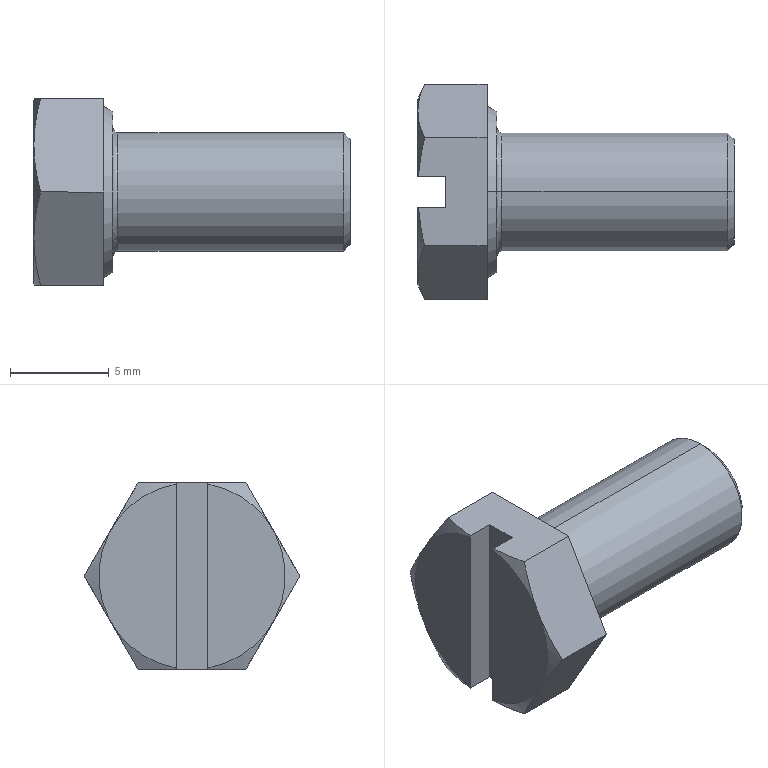Part | SolidWorks | features Cut 2, Chamfer 1, Extrusion 1, Fillet 1, LPattern 1, MoveCopyBody 1, RevCut 1, Revolution 1 | 1 solid | 24 faces | box 16 x 10.9 x 9.44 mm | volume 614.542 mm3 | plane 14 | cone 6 | torus 2 | cylinder 2 | commonest cylinder face diameters 6 x2
STEP:
#1=CARTESIAN_POINT('',(5.65,0.,-9.517));
#2=VERTEX_POINT('',#1);
#3=CARTESIAN_POINT('',(5.65,0.,-4.183));
#4=VERTEX_POINT('',#3);
#5=CARTESIAN_POINT('',(5.65,0.,-6.85));
#6=DIRECTION('',(1.,0.,0.));
#7=DIRECTION('',(0.,0.,1.));
#8=AXIS2_PLACEMENT_3D('',#5,#6,#7);
#9=CIRCLE('',#8,2.667);
#10=EDGE_CURVE('',#2,#4,#9,.T.);
#11=ORIENTED_EDGE('',*,*,#10,.F.);
#12=CARTESIAN_POINT('',(5.317,0.,-9.85));
#13=VERTEX_POINT('',#12);
#14=CARTESIAN_POINT('',(5.317,0.,-9.85));
#15=DIRECTION('',(-0.7071,0.,-0.7071));
#16=VECTOR('',#15,1000.);
#17=LINE('',#14,#16);
#18=EDGE_CURVE('',#2,#13,#17,.T.);
#19=ORIENTED_EDGE('',*,*,#18,.T.);
#20=CARTESIAN_POINT('',(5.317,0.,-3.85));
#21=VERTEX_POINT('',#20);
#22=CARTESIAN_POINT('',(5.317,0.,-6.85));
#23=DIRECTION('',(-1.,0.,0.));
#24=DIRECTION('',(0.,0.,1.));
#25=AXIS2_PLACEMENT_3D('',#22,#23,#24);
#26=CIRCLE('',#25,3.);
#27=EDGE_CURVE('',#21,#13,#26,.T.);
#28=ORIENTED_EDGE('',*,*,#27,.F.);
#29=CARTESIAN_POINT('',(5.317,0.,-3.85));
#30=DIRECTION('',(-0.7071,0.,0.7071));
#31=VECTOR('',#30,1000.);
#32=LINE('',#29,#31);
#33=EDGE_CURVE('',#4,#21,#32,.T.);
#34=ORIENTED_EDGE('',*,*,#33,.F.);
#35=EDGE_LOOP('',(#11,#19,#28,#34));
#36=FACE_OUTER_BOUND('',#35,.T.);
#37=CARTESIAN_POINT('',(5.317,0.,-6.85));
#38=DIRECTION('',(-1.,0.,0.));
#39=DIRECTION('',(0.,0.,1.));
#40=AXIS2_PLACEMENT_3D('',#37,#38,#39);
#41=CONICAL_SURFACE('',#40,3.,0.7854);
#42=ADVANCED_FACE('',(#36),#41,.T.);
#43=CARTESIAN_POINT('',(-6.35,0.,-10.1));
#44=VERTEX_POINT('',#43);
#45=CARTESIAN_POINT('',(-6.35,0.,-3.6));
#46=VERTEX_POINT('',#45);
#47=CARTESIAN_POINT('',(-6.35,0.,-6.85));
#48=DIRECTION('',(-1.,0.,0.));
#49=DIRECTION('',(0.,0.,1.));
#50=AXIS2_PLACEMENT_3D('',#47,#48,#49);
#51=CIRCLE('',#50,3.25);
#52=EDGE_CURVE('',#44,#46,#51,.T.);
#53=ORIENTED_EDGE('',*,*,#52,.F.);
#54=CARTESIAN_POINT('',(-6.1,0.,-9.85));
#55=VERTEX_POINT('',#54);
#56=CARTESIAN_POINT('',(-6.1,0.,-10.1));
#57=DIRECTION('',(0.,1.,0.));
#58=DIRECTION('',(0.,0.,1.));
#59=AXIS2_PLACEMENT_3D('',#56,#57,#58);
#60=CIRCLE('',#59,0.25);
#61=EDGE_CURVE('',#44,#55,#60,.T.);
#62=ORIENTED_EDGE('',*,*,#61,.T.);
#63=CARTESIAN_POINT('',(-6.1,0.,-3.85));
#64=VERTEX_POINT('',#63);
#65=CARTESIAN_POINT('',(-6.1,0.,-6.85));
#66=DIRECTION('',(1.,0.,0.));
#67=DIRECTION('',(0.,0.,1.));
#68=AXIS2_PLACEMENT_3D('',#65,#66,#67);
#69=CIRCLE('',#68,3.);
#70=EDGE_CURVE('',#64,#55,#69,.T.);
#71=ORIENTED_EDGE('',*,*,#70,.F.);
#72=CARTESIAN_POINT('',(-6.1,0.,-3.6));
#73=DIRECTION('',(0.,-1.,0.));
#74=DIRECTION('',(0.,0.,-1.));
#75=AXIS2_PLACEMENT_3D('',#72,#73,#74);
#76=CIRCLE('',#75,0.25);
#77=EDGE_CURVE('',#46,#64,#76,.T.);
#78=ORIENTED_EDGE('',*,*,#77,.F.);
#79=EDGE_LOOP('',(#53,#62,#71,#78));
#80=FACE_OUTER_BOUND('',#79,.T.);
#81=CARTESIAN_POINT('',(-6.1,0.,-6.85));
#82=DIRECTION('',(-1.,0.,0.));
#83=DIRECTION('',(0.,0.,1.));
#84=AXIS2_PLACEMENT_3D('',#81,#82,#83);
#85=TOROIDAL_SURFACE('',#84,3.25,0.25);
#86=ADVANCED_FACE('',(#80),#85,.F.);
#87=CARTESIAN_POINT('',(-6.35,0.,-2.789));
#88=VERTEX_POINT('',#87);
#89=CARTESIAN_POINT('',(-6.35,0.,-10.911));
#90=VERTEX_POINT('',#89);
#91=CARTESIAN_POINT('',(-6.35,0.,-6.85));
#92=DIRECTION('',(-1.,0.,0.));
#93=DIRECTION('',(0.,0.,1.));
#94=AXIS2_PLACEMENT_3D('',#91,#92,#93);
#95=CIRCLE('',#94,4.061);
#96=EDGE_CURVE('',#88,#90,#95,.T.);
#97=ORIENTED_EDGE('',*,*,#96,.T.);
#98=CARTESIAN_POINT('',(-6.85,0.,-11.2));
#99=VERTEX_POINT('',#98);
#100=CARTESIAN_POINT('',(-6.35,0.,-10.911));
#101=DIRECTION('',(-0.866,0.,-0.5));
#102=VECTOR('',#101,1000.);
#103=LINE('',#100,#102);
#104=EDGE_CURVE('',#90,#99,#103,.T.);
#105=ORIENTED_EDGE('',*,*,#104,.T.);
#106=CARTESIAN_POINT('',(-6.85,0.,-2.5));
#107=VERTEX_POINT('',#106);
#108=CARTESIAN_POINT('',(-6.85,0.,-6.85));
#109=DIRECTION('',(1.,0.,0.));
#110=DIRECTION('',(0.,0.,1.));
#111=AXIS2_PLACEMENT_3D('',#108,#109,#110);
#112=CIRCLE('',#111,4.35);
#113=EDGE_CURVE('',#99,#107,#112,.T.);
#114=ORIENTED_EDGE('',*,*,#113,.T.);
#115=CARTESIAN_POINT('',(-6.35,0.,-2.789));
#116=DIRECTION('',(-0.866,0.,0.5));
#117=VECTOR('',#116,1000.);
#118=LINE('',#115,#117);
#119=EDGE_CURVE('',#88,#107,#118,.T.);
#120=ORIENTED_EDGE('',*,*,#119,.F.);
#121=EDGE_LOOP('',(#97,#105,#114,#120));
#122=FACE_OUTER_BOUND('',#121,.T.);
#123=CARTESIAN_POINT('',(-6.35,0.,-6.85));
#124=DIRECTION('',(-1.,0.,0.));
#125=DIRECTION('',(0.,0.,1.));
#126=AXIS2_PLACEMENT_3D('',#123,#124,#125);
#127=CONICAL_SURFACE('',#126,4.061,0.5236);
#128=ADVANCED_FACE('',(#122),#127,.T.);
#129=ORIENTED_EDGE('',*,*,#27,.T.);
#130=CARTESIAN_POINT('',(-6.85,0.,-9.85));
#131=DIRECTION('',(-1.,0.,0.));
#132=VECTOR('',#131,1000.);
#133=LINE('',#130,#132);
#134=EDGE_CURVE('',#13,#55,#133,.T.);
#135=ORIENTED_EDGE('',*,*,#134,.T.);
#136=CARTESIAN_POINT('',(-6.1,0.,-6.85));
#137=DIRECTION('',(1.,0.,0.));
#138=DIRECTION('',(0.,0.,1.));
#139=AXIS2_PLACEMENT_3D('',#136,#137,#138);
#140=CIRCLE('',#139,3.);
#141=EDGE_CURVE('',#55,#64,#140,.T.);
#142=ORIENTED_EDGE('',*,*,#141,.T.);
#143=CARTESIAN_POINT('',(-6.85,0.,-3.85));
#144=DIRECTION('',(-1.,0.,0.));
#145=VECTOR('',#144,1000.);
#146=LINE('',#143,#145);
#147=EDGE_CURVE('',#21,#64,#146,.T.);
#148=ORIENTED_EDGE('',*,*,#147,.F.);
#149=EDGE_LOOP('',(#129,#135,#142,#148));
#150=FACE_OUTER_BOUND('',#149,.T.);
#151=CARTESIAN_POINT('',(-6.85,0.,-6.85));
#152=DIRECTION('',(-1.,0.,0.));
#153=DIRECTION('',(0.,0.,1.));
#154=AXIS2_PLACEMENT_3D('',#151,#152,#153);
#155=CYLINDRICAL_SURFACE('',#154,3.);
#156=ADVANCED_FACE('',(#150),#155,.T.);
#157=CARTESIAN_POINT('',(-10.319,-0.8,-11.57));
#158=VERTEX_POINT('',#157);
#159=CARTESIAN_POINT('',(-10.35,-0.8,-11.501));
#160=VERTEX_POINT('',#159);
#161=CARTESIAN_POINT('',(-10.319,-0.8,-11.57));
#162=CARTESIAN_POINT('',(-10.329,-0.8,-11.547));
#163=CARTESIAN_POINT('',(-10.34,-0.8,-11.524));
#164=CARTESIAN_POINT('',(-10.35,-0.8,-11.501));
#165=B_SPLINE_CURVE_WITH_KNOTS('',3,(#161,#162,#163,#164),.UNSPECIFIED.,.F.,.F.,(4,4),(0.006283,0.006358),.UNSPECIFIED.);
#166=EDGE_CURVE('',#158,#160,#165,.T.);
#167=ORIENTED_EDGE('',*,*,#166,.F.);
#168=CARTESIAN_POINT('',(-10.009,-2.725,-11.57));
#169=VERTEX_POINT('',#168);
#170=CARTESIAN_POINT('',(-10.319,-0.8,-11.57));
#171=CARTESIAN_POINT('',(-10.293,-1.122,-11.57));
#172=CARTESIAN_POINT('',(-10.254,-1.444,-11.57));
#173=CARTESIAN_POINT('',(-10.149,-2.086,-11.57));
#174=CARTESIAN_POINT('',(-10.083,-2.408,-11.57));
#175=CARTESIAN_POINT('',(-10.009,-2.725,-11.57));
#176=B_SPLINE_CURVE_WITH_KNOTS('',3,(#170,#171,#172,#173,#174,#175),.UNSPECIFIED.,.F.,.F.,(4,2,4),(0.01518,0.01614,0.0171),.UNSPECIFIED.);
#177=EDGE_CURVE('',#158,#169,#176,.T.);
#178=ORIENTED_EDGE('',*,*,#177,.T.);
#179=CARTESIAN_POINT('',(-10.009,-5.45,-6.85));
#180=VERTEX_POINT('',#179);
#181=CARTESIAN_POINT('',(-10.009,-2.725,-11.57));
#182=CARTESIAN_POINT('',(-10.219,-3.174,-10.792));
#183=CARTESIAN_POINT('',(-10.349,-3.626,-10.01));
#184=CARTESIAN_POINT('',(-10.35,-4.309,-8.826));
#185=CARTESIAN_POINT('',(-10.32,-4.539,-8.428));
#186=CARTESIAN_POINT('',(-10.201,-4.998,-7.633));
#187=CARTESIAN_POINT('',(-10.115,-5.225,-7.24));
#188=CARTESIAN_POINT('',(-10.009,-5.45,-6.85));
#189=B_SPLINE_CURVE_WITH_KNOTS('',3,(#181,#182,#183,#184,#185,#186,#187,#188),.UNSPECIFIED.,.F.,.F.,(4,2,2,4),(0.000000234,0.00273,0.004094,0.005459),.UNSPECIFIED.);
#190=EDGE_CURVE('',#169,#180,#189,.T.);
#191=ORIENTED_EDGE('',*,*,#190,.T.);
#192=CARTESIAN_POINT('',(-10.009,-2.725,-2.13));
#193=VERTEX_POINT('',#192);
#194=CARTESIAN_POINT('',(-10.009,-5.45,-6.85));
#195=CARTESIAN_POINT('',(-10.219,-5.001,-6.072));
#196=CARTESIAN_POINT('',(-10.349,-4.549,-5.29));
#197=CARTESIAN_POINT('',(-10.35,-3.866,-4.106));
#198=CARTESIAN_POINT('',(-10.32,-3.636,-3.708));
#199=CARTESIAN_POINT('',(-10.201,-3.177,-2.914));
#200=CARTESIAN_POINT('',(-10.115,-2.95,-2.52));
#201=CARTESIAN_POINT('',(-10.009,-2.725,-2.13));
#202=B_SPLINE_CURVE_WITH_KNOTS('',3,(#194,#195,#196,#197,#198,#199,#200,#201),.UNSPECIFIED.,.F.,.F.,(4,2,2,4),(0.000000234,0.00273,0.004094,0.005459),.UNSPECIFIED.);
#203=EDGE_CURVE('',#180,#193,#202,.T.);
#204=ORIENTED_EDGE('',*,*,#203,.T.);
#205=CARTESIAN_POINT('',(-10.319,-0.8,-2.13));
#206=VERTEX_POINT('',#205);
#207=CARTESIAN_POINT('',(-10.009,-2.725,-2.13));
#208=CARTESIAN_POINT('',(-10.083,-2.408,-2.13));
#209=CARTESIAN_POINT('',(-10.149,-2.086,-2.13));
#210=CARTESIAN_POINT('',(-10.254,-1.444,-2.13));
#211=CARTESIAN_POINT('',(-10.293,-1.122,-2.13));
#212=CARTESIAN_POINT('',(-10.319,-0.8,-2.13));
#213=B_SPLINE_CURVE_WITH_KNOTS('',3,(#207,#208,#209,#210,#211,#212),.UNSPECIFIED.,.F.,.F.,(4,2,4),(0.004915,0.00589,0.006864),.UNSPECIFIED.);
#214=EDGE_CURVE('',#193,#206,#213,.T.);
#215=ORIENTED_EDGE('',*,*,#214,.T.);
#216=CARTESIAN_POINT('',(-10.35,-0.8,-2.199));
#217=VERTEX_POINT('',#216);
#218=CARTESIAN_POINT('',(-10.35,-0.8,-2.199));
#219=CARTESIAN_POINT('',(-10.34,-0.8,-2.176));
#220=CARTESIAN_POINT('',(-10.329,-0.8,-2.153));
#221=CARTESIAN_POINT('',(-10.319,-0.8,-2.13));
#222=B_SPLINE_CURVE_WITH_KNOTS('',3,(#218,#219,#220,#221),.UNSPECIFIED.,.F.,.F.,(4,4),(0.01639,0.01646),.UNSPECIFIED.);
#223=EDGE_CURVE('',#217,#206,#222,.T.);
#224=ORIENTED_EDGE('',*,*,#223,.F.);
#225=CARTESIAN_POINT('',(-10.35,0.,-6.85));
#226=DIRECTION('',(-1.,0.,0.));
#227=DIRECTION('',(0.,0.,1.));
#228=AXIS2_PLACEMENT_3D('',#225,#226,#227);
#229=CIRCLE('',#228,4.72);
#230=EDGE_CURVE('',#160,#217,#229,.T.);
#231=ORIENTED_EDGE('',*,*,#230,.F.);
#232=EDGE_LOOP('',(#167,#178,#191,#204,#215,#224,#231));
#233=FACE_OUTER_BOUND('',#232,.T.);
#234=CARTESIAN_POINT('',(-10.35,0.,-6.85));
#235=DIRECTION('',(1.,0.,0.));
#236=DIRECTION('',(0.,0.,1.));
#237=AXIS2_PLACEMENT_3D('',#234,#235,#236);
#238=CONICAL_SURFACE('',#237,4.72,1.134);
#239=ADVANCED_FACE('',(#233),#238,.T.);
#240=CARTESIAN_POINT('',(-10.35,-0.8,-11.57));
#241=DIRECTION('',(0.,0.,1.));
#242=VECTOR('',#241,1000.);
#243=LINE('',#240,#242);
#244=EDGE_CURVE('',#160,#217,#243,.T.);
#245=ORIENTED_EDGE('',*,*,#244,.F.);
#246=ORIENTED_EDGE('',*,*,#230,.T.);
#247=EDGE_LOOP('',(#245,#246));
#248=FACE_OUTER_BOUND('',#247,.T.);
#249=CARTESIAN_POINT('',(-10.35,8.175,-11.57));
#250=DIRECTION('',(-1.,0.,0.));
#251=DIRECTION('',(0.,0.,1.));
#252=AXIS2_PLACEMENT_3D('',#249,#250,#251);
#253=PLANE('',#252);
#254=ADVANCED_FACE('',(#248),#253,.T.);
#255=CARTESIAN_POINT('',(-6.85,2.725,-2.13));
#256=VERTEX_POINT('',#255);
#257=CARTESIAN_POINT('',(-6.85,5.45,-6.85));
#258=VERTEX_POINT('',#257);
#259=CARTESIAN_POINT('',(-6.85,2.725,-2.13));
#260=DIRECTION('',(0.,0.5,-0.866));
#261=VECTOR('',#260,1000.);
#262=LINE('',#259,#261);
#263=EDGE_CURVE('',#256,#258,#262,.T.);
#264=ORIENTED_EDGE('',*,*,#263,.F.);
#265=CARTESIAN_POINT('',(-6.85,-2.725,-2.13));
#266=VERTEX_POINT('',#265);
#267=CARTESIAN_POINT('',(-6.85,-2.725,-2.13));
#268=DIRECTION('',(0.,1.,0.));
#269=VECTOR('',#268,1000.);
#270=LINE('',#267,#269);
#271=EDGE_CURVE('',#266,#256,#270,.T.);
#272=ORIENTED_EDGE('',*,*,#271,.F.);
#273=CARTESIAN_POINT('',(-6.85,-5.45,-6.85));
#274=VERTEX_POINT('',#273);
#275=CARTESIAN_POINT('',(-6.85,-5.45,-6.85));
#276=DIRECTION('',(0.,0.5,0.866));
#277=VECTOR('',#276,1000.);
#278=LINE('',#275,#277);
#279=EDGE_CURVE('',#274,#266,#278,.T.);
#280=ORIENTED_EDGE('',*,*,#279,.F.);
#281=CARTESIAN_POINT('',(-6.85,-2.725,-11.57));
#282=VERTEX_POINT('',#281);
#283=CARTESIAN_POINT('',(-6.85,-2.725,-11.57));
#284=DIRECTION('',(0.,-0.5,0.866));
#285=VECTOR('',#284,1000.);
#286=LINE('',#283,#285);
#287=EDGE_CURVE('',#282,#274,#286,.T.);
#288=ORIENTED_EDGE('',*,*,#287,.F.);
#289=CARTESIAN_POINT('',(-6.85,2.725,-11.57));
#290=VERTEX_POINT('',#289);
#291=CARTESIAN_POINT('',(-6.85,2.725,-11.57));
#292=DIRECTION('',(0.,-1.,0.));
#293=VECTOR('',#292,1000.);
#294=LINE('',#291,#293);
#295=EDGE_CURVE('',#290,#282,#294,.T.);
#296=ORIENTED_EDGE('',*,*,#295,.F.);
#297=CARTESIAN_POINT('',(-6.85,5.45,-6.85));
#298=DIRECTION('',(0.,-0.5,-0.866));
#299=VECTOR('',#298,1000.);
#300=LINE('',#297,#299);
#301=EDGE_CURVE('',#258,#290,#300,.T.);
#302=ORIENTED_EDGE('',*,*,#301,.F.);
#303=EDGE_LOOP('',(#264,#272,#280,#288,#296,#302));
#304=FACE_OUTER_BOUND('',#303,.T.);
#305=CARTESIAN_POINT('',(-6.85,0.,-6.85));
#306=DIRECTION('',(1.,0.,0.));
#307=DIRECTION('',(0.,0.,1.));
#308=AXIS2_PLACEMENT_3D('',#305,#306,#307);
#309=CIRCLE('',#308,4.35);
#310=EDGE_CURVE('',#107,#99,#309,.T.);
#311=ORIENTED_EDGE('',*,*,#310,.F.);
#312=ORIENTED_EDGE('',*,*,#113,.F.);
#313=EDGE_LOOP('',(#311,#312));
#314=FACE_BOUND('',#313,.T.);
#315=CARTESIAN_POINT('',(-6.85,8.175,-11.57));
#316=DIRECTION('',(-1.,0.,0.));
#317=DIRECTION('',(0.,0.,1.));
#318=AXIS2_PLACEMENT_3D('',#315,#316,#317);
#319=PLANE('',#318);
#320=ADVANCED_FACE('',(#304,#314),#319,.F.);
#321=CARTESIAN_POINT('',(-10.009,2.725,-2.13));
#322=VERTEX_POINT('',#321);
#323=CARTESIAN_POINT('',(-10.009,5.45,-6.85));
#324=VERTEX_POINT('',#323);
#325=CARTESIAN_POINT('',(-10.009,2.725,-2.13));
#326=CARTESIAN_POINT('',(-10.219,3.174,-2.908));
#327=CARTESIAN_POINT('',(-10.349,3.626,-3.69));
#328=CARTESIAN_POINT('',(-10.35,4.309,-4.874));
#329=CARTESIAN_POINT('',(-10.32,4.539,-5.272));
#330=CARTESIAN_POINT('',(-10.201,4.998,-6.067));
#331=CARTESIAN_POINT('',(-10.115,5.225,-6.46));
#332=CARTESIAN_POINT('',(-10.009,5.45,-6.85));
#333=B_SPLINE_CURVE_WITH_KNOTS('',3,(#325,#326,#327,#328,#329,#330,#331,#332),.UNSPECIFIED.,.F.,.F.,(4,2,2,4),(0.000000234,0.00273,0.004094,0.005459),.UNSPECIFIED.);
#334=EDGE_CURVE('',#322,#324,#333,.T.);
#335=ORIENTED_EDGE('',*,*,#334,.F.);
#336=CARTESIAN_POINT('',(-10.35,2.725,-2.13));
#337=DIRECTION('',(1.,0.,0.));
#338=VECTOR('',#337,1000.);
#339=LINE('',#336,#338);
#340=EDGE_CURVE('',#322,#256,#339,.T.);
#341=ORIENTED_EDGE('',*,*,#340,.T.);
#342=ORIENTED_EDGE('',*,*,#263,.T.);
#343=CARTESIAN_POINT('',(-10.35,5.45,-6.85));
#344=DIRECTION('',(1.,0.,0.));
#345=VECTOR('',#344,1000.);
#346=LINE('',#343,#345);
#347=EDGE_CURVE('',#324,#258,#346,.T.);
#348=ORIENTED_EDGE('',*,*,#347,.F.);
#349=EDGE_LOOP('',(#335,#341,#342,#348));
#350=FACE_OUTER_BOUND('',#349,.T.);
#351=CARTESIAN_POINT('',(-10.35,2.725,-2.13));
#352=DIRECTION('',(0.,-0.866,-0.5));
#353=DIRECTION('',(0.,-0.5,0.866));
#354=AXIS2_PLACEMENT_3D('',#351,#352,#353);
#355=PLANE('',#354);
#356=ADVANCED_FACE('',(#350),#355,.F.);
#357=CARTESIAN_POINT('',(-10.009,2.725,-11.57));
#358=VERTEX_POINT('',#357);
#359=CARTESIAN_POINT('',(-10.009,5.45,-6.85));
#360=CARTESIAN_POINT('',(-10.219,5.001,-7.628));
#361=CARTESIAN_POINT('',(-10.349,4.549,-8.41));
#362=CARTESIAN_POINT('',(-10.35,3.866,-9.594));
#363=CARTESIAN_POINT('',(-10.32,3.636,-9.992));
#364=CARTESIAN_POINT('',(-10.201,3.177,-10.786));
#365=CARTESIAN_POINT('',(-10.115,2.95,-11.18));
#366=CARTESIAN_POINT('',(-10.009,2.725,-11.57));
#367=B_SPLINE_CURVE_WITH_KNOTS('',3,(#359,#360,#361,#362,#363,#364,#365,#366),.UNSPECIFIED.,.F.,.F.,(4,2,2,4),(0.000000234,0.00273,0.004094,0.005459),.UNSPECIFIED.);
#368=EDGE_CURVE('',#324,#358,#367,.T.);
#369=ORIENTED_EDGE('',*,*,#368,.F.);
#370=ORIENTED_EDGE('',*,*,#347,.T.);
#371=ORIENTED_EDGE('',*,*,#301,.T.);
#372=CARTESIAN_POINT('',(-10.35,2.725,-11.57));
#373=DIRECTION('',(1.,0.,0.));
#374=VECTOR('',#373,1000.);
#375=LINE('',#372,#374);
#376=EDGE_CURVE('',#358,#290,#375,.T.);
#377=ORIENTED_EDGE('',*,*,#376,.F.);
#378=EDGE_LOOP('',(#369,#370,#371,#377));
#379=FACE_OUTER_BOUND('',#378,.T.);
#380=CARTESIAN_POINT('',(-10.35,5.45,-6.85));
#381=DIRECTION('',(0.,-0.866,0.5));
#382=DIRECTION('',(0.,0.5,0.866));
#383=AXIS2_PLACEMENT_3D('',#380,#381,#382);
#384=PLANE('',#383);
#385=ADVANCED_FACE('',(#379),#384,.F.);
#386=ORIENTED_EDGE('',*,*,#177,.F.);
#387=CARTESIAN_POINT('',(-8.95,-0.8,-11.57));
#388=VERTEX_POINT('',#387);
#389=CARTESIAN_POINT('',(-8.95,-0.8,-11.57));
#390=DIRECTION('',(-1.,0.,0.));
#391=VECTOR('',#390,1000.);
#392=LINE('',#389,#391);
#393=EDGE_CURVE('',#388,#158,#392,.T.);
#394=ORIENTED_EDGE('',*,*,#393,.F.);
#395=CARTESIAN_POINT('',(-8.95,0.8,-11.57));
#396=VERTEX_POINT('',#395);
#397=CARTESIAN_POINT('',(-8.95,0.8,-11.57));
#398=DIRECTION('',(0.,-1.,0.));
#399=VECTOR('',#398,1000.);
#400=LINE('',#397,#399);
#401=EDGE_CURVE('',#396,#388,#400,.T.);
#402=ORIENTED_EDGE('',*,*,#401,.F.);
#403=CARTESIAN_POINT('',(-10.319,0.8,-11.57));
#404=VERTEX_POINT('',#403);
#405=CARTESIAN_POINT('',(-8.95,0.8,-11.57));
#406=DIRECTION('',(-1.,0.,0.));
#407=VECTOR('',#406,1000.);
#408=LINE('',#405,#407);
#409=EDGE_CURVE('',#396,#404,#408,.T.);
#410=ORIENTED_EDGE('',*,*,#409,.T.);
#411=CARTESIAN_POINT('',(-10.009,2.725,-11.57));
#412=CARTESIAN_POINT('',(-10.083,2.41,-11.57));
#413=CARTESIAN_POINT('',(-10.147,2.093,-11.57));
#414=CARTESIAN_POINT('',(-10.253,1.449,-11.57));
#415=CARTESIAN_POINT('',(-10.293,1.123,-11.57));
#416=CARTESIAN_POINT('',(-10.319,0.8,-11.57));
#417=B_SPLINE_CURVE_WITH_KNOTS('',3,(#411,#412,#413,#414,#415,#416),.UNSPECIFIED.,.F.,.F.,(4,2,4),(0.01167,0.01263,0.01359),.UNSPECIFIED.);
#418=EDGE_CURVE('',#358,#404,#417,.T.);
#419=ORIENTED_EDGE('',*,*,#418,.F.);
#420=ORIENTED_EDGE('',*,*,#376,.T.);
#421=ORIENTED_EDGE('',*,*,#295,.T.);
#422=CARTESIAN_POINT('',(-10.35,-2.725,-11.57));
#423=DIRECTION('',(1.,0.,0.));
#424=VECTOR('',#423,1000.);
#425=LINE('',#422,#424);
#426=EDGE_CURVE('',#169,#282,#425,.T.);
#427=ORIENTED_EDGE('',*,*,#426,.F.);
#428=EDGE_LOOP('',(#386,#394,#402,#410,#419,#420,#421,#427));
#429=FACE_OUTER_BOUND('',#428,.T.);
#430=CARTESIAN_POINT('',(-10.35,2.725,-11.57));
#431=DIRECTION('',(0.,0.,1.));
#432=DIRECTION('',(0.,1.,0.));
#433=AXIS2_PLACEMENT_3D('',#430,#431,#432);
#434=PLANE('',#433);
#435=ADVANCED_FACE('',(#429),#434,.F.);
#436=ORIENTED_EDGE('',*,*,#190,.F.);
#437=ORIENTED_EDGE('',*,*,#426,.T.);
#438=ORIENTED_EDGE('',*,*,#287,.T.);
#439=CARTESIAN_POINT('',(-10.35,-5.45,-6.85));
#440=DIRECTION('',(1.,0.,0.));
#441=VECTOR('',#440,1000.);
#442=LINE('',#439,#441);
#443=EDGE_CURVE('',#180,#274,#442,.T.);
#444=ORIENTED_EDGE('',*,*,#443,.F.);
#445=EDGE_LOOP('',(#436,#437,#438,#444));
#446=FACE_OUTER_BOUND('',#445,.T.);
#447=CARTESIAN_POINT('',(-10.35,-2.725,-11.57));
#448=DIRECTION('',(0.,0.866,0.5));
#449=DIRECTION('',(0.,0.5,-0.866));
#450=AXIS2_PLACEMENT_3D('',#447,#448,#449);
#451=PLANE('',#450);
#452=ADVANCED_FACE('',(#446),#451,.F.);
#453=ORIENTED_EDGE('',*,*,#203,.F.);
#454=ORIENTED_EDGE('',*,*,#443,.T.);
#455=ORIENTED_EDGE('',*,*,#279,.T.);
#456=CARTESIAN_POINT('',(-10.35,-2.725,-2.13));
#457=DIRECTION('',(1.,0.,0.));
#458=VECTOR('',#457,1000.);
#459=LINE('',#456,#458);
#460=EDGE_CURVE('',#193,#266,#459,.T.);
#461=ORIENTED_EDGE('',*,*,#460,.F.);
#462=EDGE_LOOP('',(#453,#454,#455,#461));
#463=FACE_OUTER_BOUND('',#462,.T.);
#464=CARTESIAN_POINT('',(-10.35,-5.45,-6.85));
#465=DIRECTION('',(0.,0.866,-0.5));
#466=DIRECTION('',(0.,-0.5,-0.866));
#467=AXIS2_PLACEMENT_3D('',#464,#465,#466);
#468=PLANE('',#467);
#469=ADVANCED_FACE('',(#463),#468,.F.);
#470=CARTESIAN_POINT('',(-8.95,-0.8,-2.13));
#471=VERTEX_POINT('',#470);
#472=CARTESIAN_POINT('',(-8.95,0.8,-2.13));
#473=VERTEX_POINT('',#472);
#474=CARTESIAN_POINT('',(-8.95,-0.8,-2.13));
#475=DIRECTION('',(0.,1.,0.));
#476=VECTOR('',#475,1000.);
#477=LINE('',#474,#476);
#478=EDGE_CURVE('',#471,#473,#477,.T.);
#479=ORIENTED_EDGE('',*,*,#478,.F.);
#480=CARTESIAN_POINT('',(-8.95,-0.8,-2.13));
#481=DIRECTION('',(-1.,0.,0.));
#482=VECTOR('',#481,1000.);
#483=LINE('',#480,#482);
#484=EDGE_CURVE('',#471,#206,#483,.T.);
#485=ORIENTED_EDGE('',*,*,#484,.T.);
#486=ORIENTED_EDGE('',*,*,#214,.F.);
#487=ORIENTED_EDGE('',*,*,#460,.T.);
#488=ORIENTED_EDGE('',*,*,#271,.T.);
#489=ORIENTED_EDGE('',*,*,#340,.F.);
#490=CARTESIAN_POINT('',(-10.319,0.8,-2.13));
#491=VERTEX_POINT('',#490);
#492=CARTESIAN_POINT('',(-10.319,0.8,-2.13));
#493=CARTESIAN_POINT('',(-10.293,1.123,-2.13));
#494=CARTESIAN_POINT('',(-10.253,1.449,-2.13));
#495=CARTESIAN_POINT('',(-10.147,2.093,-2.13));
#496=CARTESIAN_POINT('',(-10.083,2.41,-2.13));
#497=CARTESIAN_POINT('',(-10.009,2.725,-2.13));
#498=B_SPLINE_CURVE_WITH_KNOTS('',3,(#492,#493,#494,#495,#496,#497),.UNSPECIFIED.,.F.,.F.,(4,2,4),(0.008474,0.009449,0.01042),.UNSPECIFIED.);
#499=EDGE_CURVE('',#491,#322,#498,.T.);
#500=ORIENTED_EDGE('',*,*,#499,.F.);
#501=CARTESIAN_POINT('',(-8.95,0.8,-2.13));
#502=DIRECTION('',(-1.,0.,0.));
#503=VECTOR('',#502,1000.);
#504=LINE('',#501,#503);
#505=EDGE_CURVE('',#473,#491,#504,.T.);
#506=ORIENTED_EDGE('',*,*,#505,.F.);
#507=EDGE_LOOP('',(#479,#485,#486,#487,#488,#489,#500,#506));
#508=FACE_OUTER_BOUND('',#507,.T.);
#509=CARTESIAN_POINT('',(-10.35,-2.725,-2.13));
#510=DIRECTION('',(0.,0.,-1.));
#511=DIRECTION('',(0.,-1.,0.));
#512=AXIS2_PLACEMENT_3D('',#509,#510,#511);
#513=PLANE('',#512);
#514=ADVANCED_FACE('',(#508),#513,.F.);
#515=CARTESIAN_POINT('',(-10.35,0.8,-2.199));
#516=VERTEX_POINT('',#515);
#517=CARTESIAN_POINT('',(-10.319,0.8,-2.13));
#518=CARTESIAN_POINT('',(-10.329,0.8,-2.153));
#519=CARTESIAN_POINT('',(-10.34,0.8,-2.176));
#520=CARTESIAN_POINT('',(-10.35,0.8,-2.199));
#521=B_SPLINE_CURVE_WITH_KNOTS('',3,(#517,#518,#519,#520),.UNSPECIFIED.,.F.,.F.,(4,4),(0.006283,0.006358),.UNSPECIFIED.);
#522=EDGE_CURVE('',#491,#516,#521,.T.);
#523=ORIENTED_EDGE('',*,*,#522,.F.);
#524=ORIENTED_EDGE('',*,*,#499,.T.);
#525=ORIENTED_EDGE('',*,*,#334,.T.);
#526=ORIENTED_EDGE('',*,*,#368,.T.);
#527=ORIENTED_EDGE('',*,*,#418,.T.);
#528=CARTESIAN_POINT('',(-10.35,0.8,-11.501));
#529=VERTEX_POINT('',#528);
#530=CARTESIAN_POINT('',(-10.35,0.8,-11.501));
#531=CARTESIAN_POINT('',(-10.34,0.8,-11.524));
#532=CARTESIAN_POINT('',(-10.329,0.8,-11.547));
#533=CARTESIAN_POINT('',(-10.319,0.8,-11.57));
#534=B_SPLINE_CURVE_WITH_KNOTS('',3,(#530,#531,#532,#533),.UNSPECIFIED.,.F.,.F.,(4,4),(0.01639,0.01646),.UNSPECIFIED.);
#535=EDGE_CURVE('',#529,#404,#534,.T.);
#536=ORIENTED_EDGE('',*,*,#535,.F.);
#537=CARTESIAN_POINT('',(-10.35,0.,-6.85));
#538=DIRECTION('',(-1.,0.,0.));
#539=DIRECTION('',(0.,0.,1.));
#540=AXIS2_PLACEMENT_3D('',#537,#538,#539);
#541=CIRCLE('',#540,4.72);
#542=EDGE_CURVE('',#516,#529,#541,.T.);
#543=ORIENTED_EDGE('',*,*,#542,.F.);
#544=EDGE_LOOP('',(#523,#524,#525,#526,#527,#536,#543));
#545=FACE_OUTER_BOUND('',#544,.T.);
#546=CARTESIAN_POINT('',(-10.35,0.,-6.85));
#547=DIRECTION('',(1.,0.,0.));
#548=DIRECTION('',(0.,0.,1.));
#549=AXIS2_PLACEMENT_3D('',#546,#547,#548);
#550=CONICAL_SURFACE('',#549,4.72,1.134);
#551=ADVANCED_FACE('',(#545),#550,.T.);
#552=CARTESIAN_POINT('',(-10.35,0.8,-11.57));
#553=DIRECTION('',(0.,0.,-1.));
#554=VECTOR('',#553,1000.);
#555=LINE('',#552,#554);
#556=EDGE_CURVE('',#516,#529,#555,.T.);
#557=ORIENTED_EDGE('',*,*,#556,.F.);
#558=ORIENTED_EDGE('',*,*,#542,.T.);
#559=EDGE_LOOP('',(#557,#558));
#560=FACE_OUTER_BOUND('',#559,.T.);
#561=CARTESIAN_POINT('',(-10.35,8.175,-11.57));
#562=DIRECTION('',(-1.,0.,0.));
#563=DIRECTION('',(0.,0.,1.));
#564=AXIS2_PLACEMENT_3D('',#561,#562,#563);
#565=PLANE('',#564);
#566=ADVANCED_FACE('',(#560),#565,.T.);
#567=CARTESIAN_POINT('',(-6.35,0.,-6.85));
#568=DIRECTION('',(-1.,0.,0.));
#569=DIRECTION('',(0.,0.,1.));
#570=AXIS2_PLACEMENT_3D('',#567,#568,#569);
#571=CIRCLE('',#570,3.25);
#572=EDGE_CURVE('',#46,#44,#571,.T.);
#573=ORIENTED_EDGE('',*,*,#572,.T.);
#574=ORIENTED_EDGE('',*,*,#52,.T.);
#575=EDGE_LOOP('',(#573,#574));
#576=FACE_BOUND('',#575,.T.);
#577=ORIENTED_EDGE('',*,*,#96,.F.);
#578=CARTESIAN_POINT('',(-6.35,0.,-6.85));
#579=DIRECTION('',(-1.,0.,0.));
#580=DIRECTION('',(0.,0.,1.));
#581=AXIS2_PLACEMENT_3D('',#578,#579,#580);
#582=CIRCLE('',#581,4.061);
#583=EDGE_CURVE('',#90,#88,#582,.T.);
#584=ORIENTED_EDGE('',*,*,#583,.F.);
#585=EDGE_LOOP('',(#577,#584));
#586=FACE_OUTER_BOUND('',#585,.T.);
#587=CARTESIAN_POINT('',(-6.35,3.,-6.85));
#588=DIRECTION('',(-1.,0.,0.));
#589=DIRECTION('',(0.,0.,1.));
#590=AXIS2_PLACEMENT_3D('',#587,#588,#589);
#591=PLANE('',#590);
#592=ADVANCED_FACE('',(#576,#586),#591,.F.);
#593=ORIENTED_EDGE('',*,*,#134,.F.);
#594=CARTESIAN_POINT('',(5.317,0.,-6.85));
#595=DIRECTION('',(-1.,0.,0.));
#596=DIRECTION('',(0.,0.,1.));
#597=AXIS2_PLACEMENT_3D('',#594,#595,#596);
#598=CIRCLE('',#597,3.);
#599=EDGE_CURVE('',#13,#21,#598,.T.);
#600=ORIENTED_EDGE('',*,*,#599,.T.);
#601=ORIENTED_EDGE('',*,*,#147,.T.);
#602=ORIENTED_EDGE('',*,*,#70,.T.);
#603=EDGE_LOOP('',(#593,#600,#601,#602));
#604=FACE_OUTER_BOUND('',#603,.T.);
#605=CARTESIAN_POINT('',(-6.85,0.,-6.85));
#606=DIRECTION('',(-1.,0.,0.));
#607=DIRECTION('',(0.,0.,1.));
#608=AXIS2_PLACEMENT_3D('',#605,#606,#607);
#609=CYLINDRICAL_SURFACE('',#608,3.);
#610=ADVANCED_FACE('',(#604),#609,.T.);
#611=CARTESIAN_POINT('',(5.65,0.,-6.85));
#612=DIRECTION('',(1.,0.,0.));
#613=DIRECTION('',(0.,0.,1.));
#614=AXIS2_PLACEMENT_3D('',#611,#612,#613);
#615=CIRCLE('',#614,2.667);
#616=EDGE_CURVE('',#4,#2,#615,.T.);
#617=ORIENTED_EDGE('',*,*,#616,.T.);
#618=ORIENTED_EDGE('',*,*,#10,.T.);
#619=EDGE_LOOP('',(#617,#618));
#620=FACE_OUTER_BOUND('',#619,.T.);
#621=CARTESIAN_POINT('',(5.65,3.,-6.85));
#622=DIRECTION('',(-1.,0.,0.));
#623=DIRECTION('',(0.,0.,1.));
#624=AXIS2_PLACEMENT_3D('',#621,#622,#623);
#625=PLANE('',#624);
#626=ADVANCED_FACE('',(#620),#625,.F.);
#627=ORIENTED_EDGE('',*,*,#104,.F.);
#628=ORIENTED_EDGE('',*,*,#583,.T.);
#629=ORIENTED_EDGE('',*,*,#119,.T.);
#630=ORIENTED_EDGE('',*,*,#310,.T.);
#631=EDGE_LOOP('',(#627,#628,#629,#630));
#632=FACE_OUTER_BOUND('',#631,.T.);
#633=CARTESIAN_POINT('',(-6.35,0.,-6.85));
#634=DIRECTION('',(-1.,0.,0.));
#635=DIRECTION('',(0.,0.,1.));
#636=AXIS2_PLACEMENT_3D('',#633,#634,#635);
#637=CONICAL_SURFACE('',#636,4.061,0.5236);
#638=ADVANCED_FACE('',(#632),#637,.T.);
#639=ORIENTED_EDGE('',*,*,#61,.F.);
#640=ORIENTED_EDGE('',*,*,#572,.F.);
#641=ORIENTED_EDGE('',*,*,#77,.T.);
#642=ORIENTED_EDGE('',*,*,#141,.F.);
#643=EDGE_LOOP('',(#639,#640,#641,#642));
#644=FACE_OUTER_BOUND('',#643,.T.);
#645=CARTESIAN_POINT('',(-6.1,0.,-6.85));
#646=DIRECTION('',(-1.,0.,0.));
#647=DIRECTION('',(0.,0.,1.));
#648=AXIS2_PLACEMENT_3D('',#645,#646,#647);
#649=TOROIDAL_SURFACE('',#648,3.25,0.25);
#650=ADVANCED_FACE('',(#644),#649,.F.);
#651=ORIENTED_EDGE('',*,*,#18,.F.);
#652=ORIENTED_EDGE('',*,*,#616,.F.);
#653=ORIENTED_EDGE('',*,*,#33,.T.);
#654=ORIENTED_EDGE('',*,*,#599,.F.);
#655=EDGE_LOOP('',(#651,#652,#653,#654));
#656=FACE_OUTER_BOUND('',#655,.T.);
#657=CARTESIAN_POINT('',(5.317,0.,-6.85));
#658=DIRECTION('',(-1.,0.,0.));
#659=DIRECTION('',(0.,0.,1.));
#660=AXIS2_PLACEMENT_3D('',#657,#658,#659);
#661=CONICAL_SURFACE('',#660,3.,0.7854);
#662=ADVANCED_FACE('',(#656),#661,.T.);
#663=ORIENTED_EDGE('',*,*,#166,.T.);
#664=ORIENTED_EDGE('',*,*,#244,.T.);
#665=ORIENTED_EDGE('',*,*,#223,.T.);
#666=ORIENTED_EDGE('',*,*,#484,.F.);
#667=CARTESIAN_POINT('',(-8.95,-0.8,-11.57));
#668=DIRECTION('',(0.,0.,1.));
#669=VECTOR('',#668,1000.);
#670=LINE('',#667,#669);
#671=EDGE_CURVE('',#388,#471,#670,.T.);
#672=ORIENTED_EDGE('',*,*,#671,.F.);
#673=ORIENTED_EDGE('',*,*,#393,.T.);
#674=EDGE_LOOP('',(#663,#664,#665,#666,#672,#673));
#675=FACE_OUTER_BOUND('',#674,.T.);
#676=CARTESIAN_POINT('',(-8.95,-0.8,-11.57));
#677=DIRECTION('',(0.,-1.,0.));
#678=DIRECTION('',(0.,0.,1.));
#679=AXIS2_PLACEMENT_3D('',#676,#677,#678);
#680=PLANE('',#679);
#681=ADVANCED_FACE('',(#675),#680,.F.);
#682=ORIENTED_EDGE('',*,*,#522,.T.);
#683=ORIENTED_EDGE('',*,*,#556,.T.);
#684=ORIENTED_EDGE('',*,*,#535,.T.);
#685=ORIENTED_EDGE('',*,*,#409,.F.);
#686=CARTESIAN_POINT('',(-8.95,0.8,-11.57));
#687=DIRECTION('',(0.,0.,-1.));
#688=VECTOR('',#687,1000.);
#689=LINE('',#686,#688);
#690=EDGE_CURVE('',#473,#396,#689,.T.);
#691=ORIENTED_EDGE('',*,*,#690,.F.);
#692=ORIENTED_EDGE('',*,*,#505,.T.);
#693=EDGE_LOOP('',(#682,#683,#684,#685,#691,#692));
#694=FACE_OUTER_BOUND('',#693,.T.);
#695=CARTESIAN_POINT('',(-8.95,0.8,-11.57));
#696=DIRECTION('',(0.,1.,0.));
#697=DIRECTION('',(0.,0.,-1.));
#698=AXIS2_PLACEMENT_3D('',#695,#696,#697);
#699=PLANE('',#698);
#700=ADVANCED_FACE('',(#694),#699,.F.);
#701=ORIENTED_EDGE('',*,*,#478,.T.);
#702=ORIENTED_EDGE('',*,*,#690,.T.);
#703=ORIENTED_EDGE('',*,*,#401,.T.);
#704=ORIENTED_EDGE('',*,*,#671,.T.);
#705=EDGE_LOOP('',(#701,#702,#703,#704));
#706=FACE_OUTER_BOUND('',#705,.T.);
#707=CARTESIAN_POINT('',(-8.95,0.8,-2.13));
#708=DIRECTION('',(1.,0.,0.));
#709=DIRECTION('',(0.,0.,-1.));
#710=AXIS2_PLACEMENT_3D('',#707,#708,#709);
#711=PLANE('',#710);
#712=ADVANCED_FACE('',(#706),#711,.F.);
#713=CLOSED_SHELL('',(#42,#86,#128,#156,#239,#254,#320,#356,#385,#435,#452,#469,#514,#551,#566,#592,#610,#626,#638,#650,#662,#681,#700,#712));
#714=MANIFOLD_SOLID_BREP('',#713);
#715=CARTESIAN_POINT('',(0.,0.,0.));
#716=DIRECTION('',(0.,0.,1.));
#717=DIRECTION('',(1.,0.,0.));
#718=AXIS2_PLACEMENT_3D('',#715,#716,#717);
#719=(LENGTH_UNIT()NAMED_UNIT(*)SI_UNIT(.MILLI.,.METRE.));
#720=UNCERTAINTY_MEASURE_WITH_UNIT(LENGTH_MEASURE(0.00001),#719,'','');
#721=(NAMED_UNIT(*)PLANE_ANGLE_UNIT()SI_UNIT($,.RADIAN.));
#722=(NAMED_UNIT(*)SI_UNIT($,.STERADIAN.)SOLID_ANGLE_UNIT());
#723=(GEOMETRIC_REPRESENTATION_CONTEXT(3)GLOBAL_UNCERTAINTY_ASSIGNED_CONTEXT((#720))GLOBAL_UNIT_ASSIGNED_CONTEXT((#719,#721,#722))REPRESENTATION_CONTEXT('',''));
#724=ADVANCED_BREP_SHAPE_REPRESENTATION('',(#714,#718),#723);